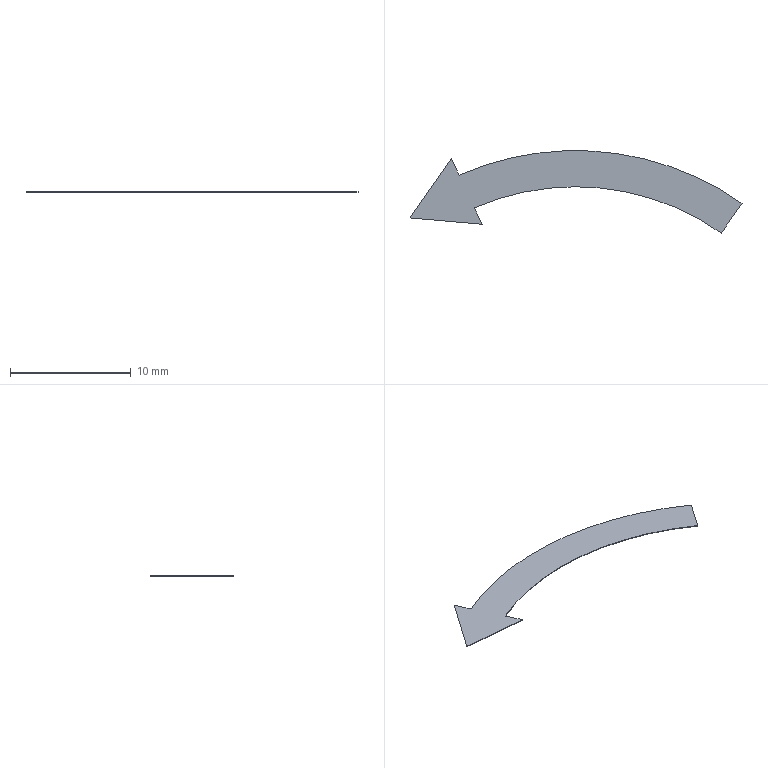Part | STEP file | J101-EBZ05-16-12-Part-1 | 1 solid | 9 faces | box 27.536 x 6.847 x 0.05 mm | volume 4.242 mm3 | plane 7 | cylinder 2 | commonest cylinder face diameters 41.852 x1 47.852 x1
STEP:
#1=CARTESIAN_POINT('',(12.234,7.825,0.05));
#2=VERTEX_POINT('',#1);
#3=CARTESIAN_POINT('',(13.955,10.283,0.05));
#4=VERTEX_POINT('',#3);
#5=CARTESIAN_POINT('',(12.234,7.825,0.05));
#6=DIRECTION('',(0.5736,0.8192,0.));
#7=VECTOR('',#6,1000.);
#8=LINE('',#5,#7);
#9=EDGE_CURVE('',#2,#4,#8,.T.);
#10=ORIENTED_EDGE('',*,*,#9,.F.);
#11=CARTESIAN_POINT('',(12.234,7.825,0.));
#12=VERTEX_POINT('',#11);
#13=CARTESIAN_POINT('',(12.234,7.825,0.));
#14=DIRECTION('',(0.,0.,1.));
#15=VECTOR('',#14,1000.);
#16=LINE('',#13,#15);
#17=EDGE_CURVE('',#12,#2,#16,.T.);
#18=ORIENTED_EDGE('',*,*,#17,.F.);
#19=CARTESIAN_POINT('',(13.955,10.283,0.));
#20=VERTEX_POINT('',#19);
#21=CARTESIAN_POINT('',(12.234,7.825,0.));
#22=DIRECTION('',(0.5736,0.8192,0.));
#23=VECTOR('',#22,1000.);
#24=LINE('',#21,#23);
#25=EDGE_CURVE('',#12,#20,#24,.T.);
#26=ORIENTED_EDGE('',*,*,#25,.T.);
#27=CARTESIAN_POINT('',(13.955,10.283,0.));
#28=DIRECTION('',(0.,0.,1.));
#29=VECTOR('',#28,1000.);
#30=LINE('',#27,#29);
#31=EDGE_CURVE('',#20,#4,#30,.T.);
#32=ORIENTED_EDGE('',*,*,#31,.T.);
#33=EDGE_LOOP('',(#10,#18,#26,#32));
#34=FACE_OUTER_BOUND('',#33,.T.);
#35=CARTESIAN_POINT('',(12.234,7.825,0.));
#36=DIRECTION('',(0.8192,-0.5736,0.));
#37=DIRECTION('',(0.5736,0.8192,0.));
#38=AXIS2_PLACEMENT_3D('',#35,#36,#37);
#39=PLANE('',#38);
#40=ADVANCED_FACE('',(#34),#39,.T.);
#41=CARTESIAN_POINT('',(-9.504,12.641,0.05));
#42=VERTEX_POINT('',#41);
#43=CARTESIAN_POINT('',(0.143,-9.254,0.05));
#44=DIRECTION('',(0.,0.,1.));
#45=DIRECTION('',(0.9962,-0.08716,0.));
#46=AXIS2_PLACEMENT_3D('',#43,#44,#45);
#47=CIRCLE('',#46,23.926);
#48=EDGE_CURVE('',#4,#42,#47,.T.);
#49=ORIENTED_EDGE('',*,*,#48,.F.);
#50=ORIENTED_EDGE('',*,*,#31,.F.);
#51=CARTESIAN_POINT('',(-9.504,12.641,0.));
#52=VERTEX_POINT('',#51);
#53=CARTESIAN_POINT('',(0.143,-9.254,0.));
#54=DIRECTION('',(0.,0.,1.));
#55=DIRECTION('',(0.9962,-0.08716,0.));
#56=AXIS2_PLACEMENT_3D('',#53,#54,#55);
#57=CIRCLE('',#56,23.926);
#58=EDGE_CURVE('',#20,#52,#57,.T.);
#59=ORIENTED_EDGE('',*,*,#58,.T.);
#60=CARTESIAN_POINT('',(-9.504,12.641,0.));
#61=DIRECTION('',(0.,0.,1.));
#62=VECTOR('',#61,1000.);
#63=LINE('',#60,#62);
#64=EDGE_CURVE('',#52,#42,#63,.T.);
#65=ORIENTED_EDGE('',*,*,#64,.T.);
#66=EDGE_LOOP('',(#49,#50,#59,#65));
#67=FACE_OUTER_BOUND('',#66,.T.);
#68=CARTESIAN_POINT('',(0.143,-9.254,0.));
#69=DIRECTION('',(0.,0.,1.));
#70=DIRECTION('',(0.9962,-0.08716,0.));
#71=AXIS2_PLACEMENT_3D('',#68,#69,#70);
#72=CYLINDRICAL_SURFACE('',#71,23.926);
#73=ADVANCED_FACE('',(#67),#72,.T.);
#74=CARTESIAN_POINT('',(-10.138,14.001,0.05));
#75=VERTEX_POINT('',#74);
#76=CARTESIAN_POINT('',(-9.504,12.641,0.05));
#77=DIRECTION('',(-0.4226,0.9063,0.));
#78=VECTOR('',#77,1000.);
#79=LINE('',#76,#78);
#80=EDGE_CURVE('',#42,#75,#79,.T.);
#81=ORIENTED_EDGE('',*,*,#80,.F.);
#82=ORIENTED_EDGE('',*,*,#64,.F.);
#83=CARTESIAN_POINT('',(-10.138,14.001,0.));
#84=VERTEX_POINT('',#83);
#85=CARTESIAN_POINT('',(-9.504,12.641,0.));
#86=DIRECTION('',(-0.4226,0.9063,0.));
#87=VECTOR('',#86,1000.);
#88=LINE('',#85,#87);
#89=EDGE_CURVE('',#52,#84,#88,.T.);
#90=ORIENTED_EDGE('',*,*,#89,.T.);
#91=CARTESIAN_POINT('',(-10.138,14.001,0.));
#92=DIRECTION('',(0.,0.,1.));
#93=VECTOR('',#92,1000.);
#94=LINE('',#91,#93);
#95=EDGE_CURVE('',#84,#75,#94,.T.);
#96=ORIENTED_EDGE('',*,*,#95,.T.);
#97=EDGE_LOOP('',(#81,#82,#90,#96));
#98=FACE_OUTER_BOUND('',#97,.T.);
#99=CARTESIAN_POINT('',(-9.504,12.641,0.));
#100=DIRECTION('',(0.9063,0.4226,0.));
#101=DIRECTION('',(-0.4226,0.9063,0.));
#102=AXIS2_PLACEMENT_3D('',#99,#100,#101);
#103=PLANE('',#102);
#104=ADVANCED_FACE('',(#98),#103,.T.);
#105=CARTESIAN_POINT('',(-13.581,9.085,0.05));
#106=VERTEX_POINT('',#105);
#107=CARTESIAN_POINT('',(-10.138,14.001,0.05));
#108=DIRECTION('',(-0.5736,-0.8192,0.));
#109=VECTOR('',#108,1000.);
#110=LINE('',#107,#109);
#111=EDGE_CURVE('',#75,#106,#110,.T.);
#112=ORIENTED_EDGE('',*,*,#111,.F.);
#113=ORIENTED_EDGE('',*,*,#95,.F.);
#114=CARTESIAN_POINT('',(-13.581,9.085,0.));
#115=VERTEX_POINT('',#114);
#116=CARTESIAN_POINT('',(-10.138,14.001,0.));
#117=DIRECTION('',(-0.5736,-0.8192,0.));
#118=VECTOR('',#117,1000.);
#119=LINE('',#116,#118);
#120=EDGE_CURVE('',#84,#115,#119,.T.);
#121=ORIENTED_EDGE('',*,*,#120,.T.);
#122=CARTESIAN_POINT('',(-13.581,9.085,0.));
#123=DIRECTION('',(0.,0.,1.));
#124=VECTOR('',#123,1000.);
#125=LINE('',#122,#124);
#126=EDGE_CURVE('',#115,#106,#125,.T.);
#127=ORIENTED_EDGE('',*,*,#126,.T.);
#128=EDGE_LOOP('',(#112,#113,#121,#127));
#129=FACE_OUTER_BOUND('',#128,.T.);
#130=CARTESIAN_POINT('',(-10.138,14.001,0.));
#131=DIRECTION('',(-0.8192,0.5736,0.));
#132=DIRECTION('',(-0.5736,-0.8192,0.));
#133=AXIS2_PLACEMENT_3D('',#130,#131,#132);
#134=PLANE('',#133);
#135=ADVANCED_FACE('',(#129),#134,.T.);
#136=CARTESIAN_POINT('',(-7.602,8.562,0.05));
#137=VERTEX_POINT('',#136);
#138=CARTESIAN_POINT('',(-13.581,9.085,0.05));
#139=DIRECTION('',(0.9962,-0.08716,0.));
#140=VECTOR('',#139,1000.);
#141=LINE('',#138,#140);
#142=EDGE_CURVE('',#106,#137,#141,.T.);
#143=ORIENTED_EDGE('',*,*,#142,.F.);
#144=ORIENTED_EDGE('',*,*,#126,.F.);
#145=CARTESIAN_POINT('',(-7.602,8.562,0.));
#146=VERTEX_POINT('',#145);
#147=CARTESIAN_POINT('',(-13.581,9.085,0.));
#148=DIRECTION('',(0.9962,-0.08716,0.));
#149=VECTOR('',#148,1000.);
#150=LINE('',#147,#149);
#151=EDGE_CURVE('',#115,#146,#150,.T.);
#152=ORIENTED_EDGE('',*,*,#151,.T.);
#153=CARTESIAN_POINT('',(-7.602,8.562,0.));
#154=DIRECTION('',(0.,0.,1.));
#155=VECTOR('',#154,1000.);
#156=LINE('',#153,#155);
#157=EDGE_CURVE('',#146,#137,#156,.T.);
#158=ORIENTED_EDGE('',*,*,#157,.T.);
#159=EDGE_LOOP('',(#143,#144,#152,#158));
#160=FACE_OUTER_BOUND('',#159,.T.);
#161=CARTESIAN_POINT('',(-13.581,9.085,0.));
#162=DIRECTION('',(-0.08716,-0.9962,0.));
#163=DIRECTION('',(0.9962,-0.08716,0.));
#164=AXIS2_PLACEMENT_3D('',#161,#162,#163);
#165=PLANE('',#164);
#166=ADVANCED_FACE('',(#160),#165,.T.);
#167=CARTESIAN_POINT('',(-8.236,9.921,0.05));
#168=VERTEX_POINT('',#167);
#169=CARTESIAN_POINT('',(-7.602,8.562,0.05));
#170=DIRECTION('',(-0.4226,0.9063,0.));
#171=VECTOR('',#170,1000.);
#172=LINE('',#169,#171);
#173=EDGE_CURVE('',#137,#168,#172,.T.);
#174=ORIENTED_EDGE('',*,*,#173,.F.);
#175=ORIENTED_EDGE('',*,*,#157,.F.);
#176=CARTESIAN_POINT('',(-8.236,9.921,0.));
#177=VERTEX_POINT('',#176);
#178=CARTESIAN_POINT('',(-7.602,8.562,0.));
#179=DIRECTION('',(-0.4226,0.9063,0.));
#180=VECTOR('',#179,1000.);
#181=LINE('',#178,#180);
#182=EDGE_CURVE('',#146,#177,#181,.T.);
#183=ORIENTED_EDGE('',*,*,#182,.T.);
#184=CARTESIAN_POINT('',(-8.236,9.921,0.));
#185=DIRECTION('',(0.,0.,1.));
#186=VECTOR('',#185,1000.);
#187=LINE('',#184,#186);
#188=EDGE_CURVE('',#177,#168,#187,.T.);
#189=ORIENTED_EDGE('',*,*,#188,.T.);
#190=EDGE_LOOP('',(#174,#175,#183,#189));
#191=FACE_OUTER_BOUND('',#190,.T.);
#192=CARTESIAN_POINT('',(-7.602,8.562,0.));
#193=DIRECTION('',(0.9063,0.4226,0.));
#194=DIRECTION('',(-0.4226,0.9063,0.));
#195=AXIS2_PLACEMENT_3D('',#192,#193,#194);
#196=PLANE('',#195);
#197=ADVANCED_FACE('',(#191),#196,.T.);
#198=CARTESIAN_POINT('',(0.143,-9.254,0.05));
#199=DIRECTION('',(0.,0.,-1.));
#200=DIRECTION('',(-0.9962,0.08716,0.));
#201=AXIS2_PLACEMENT_3D('',#198,#199,#200);
#202=CIRCLE('',#201,20.926);
#203=EDGE_CURVE('',#168,#2,#202,.T.);
#204=ORIENTED_EDGE('',*,*,#203,.F.);
#205=ORIENTED_EDGE('',*,*,#188,.F.);
#206=CARTESIAN_POINT('',(0.143,-9.254,0.));
#207=DIRECTION('',(0.,0.,-1.));
#208=DIRECTION('',(-0.9962,0.08716,0.));
#209=AXIS2_PLACEMENT_3D('',#206,#207,#208);
#210=CIRCLE('',#209,20.926);
#211=EDGE_CURVE('',#177,#12,#210,.T.);
#212=ORIENTED_EDGE('',*,*,#211,.T.);
#213=ORIENTED_EDGE('',*,*,#17,.T.);
#214=EDGE_LOOP('',(#204,#205,#212,#213));
#215=FACE_OUTER_BOUND('',#214,.T.);
#216=CARTESIAN_POINT('',(0.143,-9.254,0.));
#217=DIRECTION('',(0.,0.,1.));
#218=DIRECTION('',(0.9962,-0.08716,0.));
#219=AXIS2_PLACEMENT_3D('',#216,#217,#218);
#220=CYLINDRICAL_SURFACE('',#219,20.926);
#221=ADVANCED_FACE('',(#215),#220,.F.);
#222=ORIENTED_EDGE('',*,*,#25,.F.);
#223=ORIENTED_EDGE('',*,*,#211,.F.);
#224=ORIENTED_EDGE('',*,*,#182,.F.);
#225=ORIENTED_EDGE('',*,*,#151,.F.);
#226=ORIENTED_EDGE('',*,*,#120,.F.);
#227=ORIENTED_EDGE('',*,*,#89,.F.);
#228=ORIENTED_EDGE('',*,*,#58,.F.);
#229=EDGE_LOOP('',(#222,#223,#224,#225,#226,#227,#228));
#230=FACE_OUTER_BOUND('',#229,.T.);
#231=CARTESIAN_POINT('',(0.143,-9.254,0.));
#232=DIRECTION('',(0.,0.,1.));
#233=DIRECTION('',(0.9962,-0.08716,0.));
#234=AXIS2_PLACEMENT_3D('',#231,#232,#233);
#235=PLANE('',#234);
#236=ADVANCED_FACE('',(#230),#235,.F.);
#237=ORIENTED_EDGE('',*,*,#9,.T.);
#238=ORIENTED_EDGE('',*,*,#48,.T.);
#239=ORIENTED_EDGE('',*,*,#80,.T.);
#240=ORIENTED_EDGE('',*,*,#111,.T.);
#241=ORIENTED_EDGE('',*,*,#142,.T.);
#242=ORIENTED_EDGE('',*,*,#173,.T.);
#243=ORIENTED_EDGE('',*,*,#203,.T.);
#244=EDGE_LOOP('',(#237,#238,#239,#240,#241,#242,#243));
#245=FACE_OUTER_BOUND('',#244,.T.);
#246=CARTESIAN_POINT('',(0.143,-9.254,0.05));
#247=DIRECTION('',(0.,0.,1.));
#248=DIRECTION('',(0.9962,-0.08716,0.));
#249=AXIS2_PLACEMENT_3D('',#246,#247,#248);
#250=PLANE('',#249);
#251=ADVANCED_FACE('',(#245),#250,.T.);
#252=CLOSED_SHELL('',(#40,#73,#104,#135,#166,#197,#221,#236,#251));
#253=MANIFOLD_SOLID_BREP('',#252);
#254=CARTESIAN_POINT('',(0.,0.,0.));
#255=DIRECTION('',(0.,0.,1.));
#256=DIRECTION('',(1.,0.,0.));
#257=AXIS2_PLACEMENT_3D('',#254,#255,#256);
#258=(LENGTH_UNIT()NAMED_UNIT(*)SI_UNIT(.MILLI.,.METRE.));
#259=UNCERTAINTY_MEASURE_WITH_UNIT(LENGTH_MEASURE(0.00001),#258,'','');
#260=(NAMED_UNIT(*)PLANE_ANGLE_UNIT()SI_UNIT($,.RADIAN.));
#261=(NAMED_UNIT(*)SI_UNIT($,.STERADIAN.)SOLID_ANGLE_UNIT());
#262=(GEOMETRIC_REPRESENTATION_CONTEXT(3)GLOBAL_UNCERTAINTY_ASSIGNED_CONTEXT((#259))GLOBAL_UNIT_ASSIGNED_CONTEXT((#258,#260,#261))REPRESENTATION_CONTEXT('',''));
#263=ADVANCED_BREP_SHAPE_REPRESENTATION('',(#253,#257),#262);